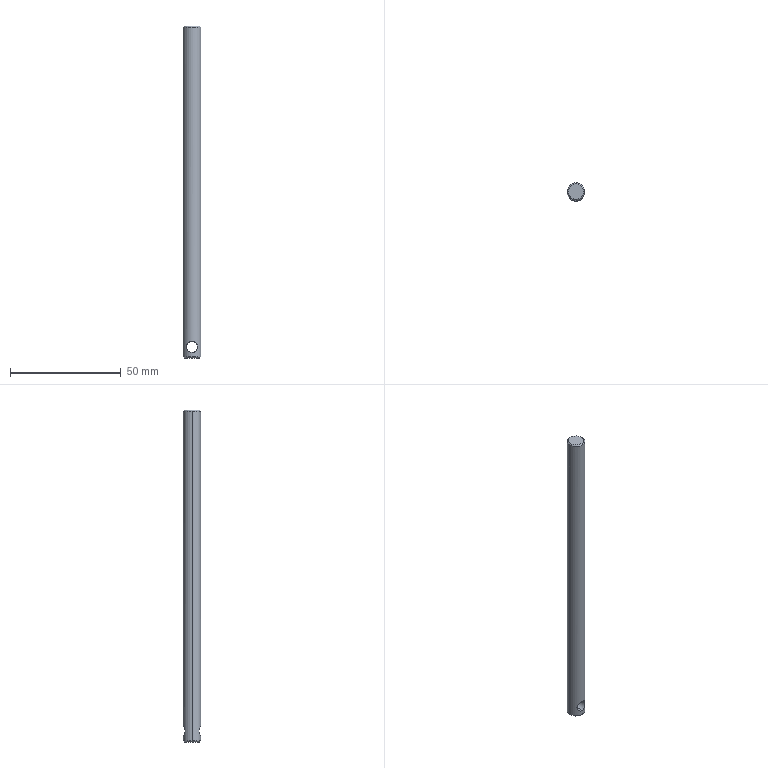Part | SolidWorks | features Chamfer 1, Extrusion 1, ICE 1 | 1 solid | 10 faces | box 8 x 8 x 150 mm | volume 7385 mm3 | cone 4 | cylinder 4 | plane 2 | commonest cylinder face diameters 5 x2 8 x2
STEP:
#1=CARTESIAN_POINT('',(-3.5,0.,-75.));
#2=VERTEX_POINT('',#1);
#3=CARTESIAN_POINT('',(3.5,0.,-75.));
#4=VERTEX_POINT('',#3);
#5=CARTESIAN_POINT('',(0.,0.,-75.));
#6=DIRECTION('',(0.,0.,-1.));
#7=DIRECTION('',(1.,0.,0.));
#8=AXIS2_PLACEMENT_3D('',#5,#6,#7);
#9=CIRCLE('',#8,3.5);
#10=EDGE_CURVE('',#2,#4,#9,.T.);
#11=ORIENTED_EDGE('',*,*,#10,.F.);
#12=CARTESIAN_POINT('',(-4.,0.,-74.5));
#13=VERTEX_POINT('',#12);
#14=CARTESIAN_POINT('',(-4.,0.,-74.5));
#15=DIRECTION('',(-0.7071,0.,0.7071));
#16=VECTOR('',#15,1000.);
#17=LINE('',#14,#16);
#18=EDGE_CURVE('',#2,#13,#17,.T.);
#19=ORIENTED_EDGE('',*,*,#18,.T.);
#20=CARTESIAN_POINT('',(4.,0.,-74.5));
#21=VERTEX_POINT('',#20);
#22=CARTESIAN_POINT('',(0.,0.,-74.5));
#23=DIRECTION('',(0.,0.,1.));
#24=DIRECTION('',(1.,0.,0.));
#25=AXIS2_PLACEMENT_3D('',#22,#23,#24);
#26=CIRCLE('',#25,4.);
#27=EDGE_CURVE('',#21,#13,#26,.T.);
#28=ORIENTED_EDGE('',*,*,#27,.F.);
#29=CARTESIAN_POINT('',(4.,0.,-74.5));
#30=DIRECTION('',(0.7071,0.,0.7071));
#31=VECTOR('',#30,1000.);
#32=LINE('',#29,#31);
#33=EDGE_CURVE('',#4,#21,#32,.T.);
#34=ORIENTED_EDGE('',*,*,#33,.F.);
#35=EDGE_LOOP('',(#11,#19,#28,#34));
#36=FACE_OUTER_BOUND('',#35,.T.);
#37=CARTESIAN_POINT('',(0.,0.,-74.5));
#38=DIRECTION('',(0.,0.,1.));
#39=DIRECTION('',(1.,0.,0.));
#40=AXIS2_PLACEMENT_3D('',#37,#38,#39);
#41=CONICAL_SURFACE('',#40,4.,0.7854);
#42=ADVANCED_FACE('',(#36),#41,.T.);
#43=CARTESIAN_POINT('',(3.5,0.,75.));
#44=VERTEX_POINT('',#43);
#45=CARTESIAN_POINT('',(-3.5,0.,75.));
#46=VERTEX_POINT('',#45);
#47=CARTESIAN_POINT('',(0.,0.,75.));
#48=DIRECTION('',(0.,0.,1.));
#49=DIRECTION('',(1.,0.,0.));
#50=AXIS2_PLACEMENT_3D('',#47,#48,#49);
#51=CIRCLE('',#50,3.5);
#52=EDGE_CURVE('',#44,#46,#51,.T.);
#53=ORIENTED_EDGE('',*,*,#52,.F.);
#54=CARTESIAN_POINT('',(4.,0.,74.5));
#55=VERTEX_POINT('',#54);
#56=CARTESIAN_POINT('',(3.5,0.,75.));
#57=DIRECTION('',(0.7071,0.,-0.7071));
#58=VECTOR('',#57,1000.);
#59=LINE('',#56,#58);
#60=EDGE_CURVE('',#44,#55,#59,.T.);
#61=ORIENTED_EDGE('',*,*,#60,.T.);
#62=CARTESIAN_POINT('',(-4.,0.,74.5));
#63=VERTEX_POINT('',#62);
#64=CARTESIAN_POINT('',(0.,0.,74.5));
#65=DIRECTION('',(0.,0.,-1.));
#66=DIRECTION('',(1.,0.,0.));
#67=AXIS2_PLACEMENT_3D('',#64,#65,#66);
#68=CIRCLE('',#67,4.);
#69=EDGE_CURVE('',#63,#55,#68,.T.);
#70=ORIENTED_EDGE('',*,*,#69,.F.);
#71=CARTESIAN_POINT('',(-3.5,0.,75.));
#72=DIRECTION('',(-0.7071,0.,-0.7071));
#73=VECTOR('',#72,1000.);
#74=LINE('',#71,#73);
#75=EDGE_CURVE('',#46,#63,#74,.T.);
#76=ORIENTED_EDGE('',*,*,#75,.F.);
#77=EDGE_LOOP('',(#53,#61,#70,#76));
#78=FACE_OUTER_BOUND('',#77,.T.);
#79=CARTESIAN_POINT('',(0.,0.,75.));
#80=DIRECTION('',(0.,0.,-1.));
#81=DIRECTION('',(-1.,0.,0.));
#82=AXIS2_PLACEMENT_3D('',#79,#80,#81);
#83=CONICAL_SURFACE('',#82,3.5,0.7854);
#84=ADVANCED_FACE('',(#78),#83,.T.);
#85=CARTESIAN_POINT('',(0.,-4.,-72.5));
#86=VERTEX_POINT('',#85);
#87=CARTESIAN_POINT('',(0.,-4.,-67.5));
#88=VERTEX_POINT('',#87);
#89=CARTESIAN_POINT('',(0.,-4.,-72.5));
#90=CARTESIAN_POINT('',(-0.1686,-4.,-72.5));
#91=CARTESIAN_POINT('',(-0.335,-3.989,-72.483));
#92=CARTESIAN_POINT('',(-0.6633,-3.948,-72.416));
#93=CARTESIAN_POINT('',(-0.8235,-3.917,-72.366));
#94=CARTESIAN_POINT('',(-1.125,-3.842,-72.239));
#95=CARTESIAN_POINT('',(-1.27,-3.796,-72.16));
#96=CARTESIAN_POINT('',(-1.536,-3.696,-71.979));
#97=CARTESIAN_POINT('',(-1.659,-3.642,-71.877));
#98=CARTESIAN_POINT('',(-1.884,-3.531,-71.651));
#99=CARTESIAN_POINT('',(-1.985,-3.474,-71.527));
#100=CARTESIAN_POINT('',(-2.163,-3.367,-71.264));
#101=CARTESIAN_POINT('',(-2.239,-3.315,-71.124));
#102=CARTESIAN_POINT('',(-2.367,-3.226,-70.822));
#103=CARTESIAN_POINT('',(-2.416,-3.189,-70.665));
#104=CARTESIAN_POINT('',(-2.482,-3.137,-70.34));
#105=CARTESIAN_POINT('',(-2.5,-3.123,-70.169));
#106=CARTESIAN_POINT('',(-2.5,-3.122,-69.834));
#107=CARTESIAN_POINT('',(-2.483,-3.136,-69.666));
#108=CARTESIAN_POINT('',(-2.416,-3.188,-69.337));
#109=CARTESIAN_POINT('',(-2.367,-3.225,-69.18));
#110=CARTESIAN_POINT('',(-2.177,-3.359,-68.729));
#111=CARTESIAN_POINT('',(-1.996,-3.476,-68.461));
#112=CARTESIAN_POINT('',(-1.659,-3.642,-68.123));
#113=CARTESIAN_POINT('',(-1.536,-3.696,-68.021));
#114=CARTESIAN_POINT('',(-1.271,-3.795,-67.841));
#115=CARTESIAN_POINT('',(-1.126,-3.841,-67.762));
#116=CARTESIAN_POINT('',(-0.8248,-3.917,-67.634));
#117=CARTESIAN_POINT('',(-0.6682,-3.947,-67.585));
#118=CARTESIAN_POINT('',(-0.3411,-3.989,-67.518));
#119=CARTESIAN_POINT('',(-0.1698,-4.,-67.5));
#120=CARTESIAN_POINT('',(0.,-4.,-67.5));
#121=B_SPLINE_CURVE_WITH_KNOTS('',3,(#89,#90,#91,#92,#93,#94,#95,#96,#97,#98,#99,#100,#101,#102,#103,#104,#105,#106,#107,#108,#109,#110,#111,#112,#113,#114,#115,#116,#117,#118,#119,#120),.UNSPECIFIED.,.F.,.F.,(4,2,2,2,2,2,2,2,2,2,2,2,2,2,2,4),(0.008042,0.008543,0.009045,0.009546,0.01005,0.01055,0.01105,0.01155,0.01205,0.01256,0.01306,0.01406,0.01456,0.01506,0.01556,0.01607),.UNSPECIFIED.);
#122=EDGE_CURVE('',#86,#88,#121,.T.);
#123=ORIENTED_EDGE('',*,*,#122,.F.);
#124=CARTESIAN_POINT('',(0.,4.,-72.5));
#125=VERTEX_POINT('',#124);
#126=CARTESIAN_POINT('',(0.,-75.,-72.5));
#127=DIRECTION('',(0.,1.,0.));
#128=VECTOR('',#127,1000.);
#129=LINE('',#126,#128);
#130=EDGE_CURVE('',#86,#125,#129,.T.);
#131=ORIENTED_EDGE('',*,*,#130,.T.);
#132=CARTESIAN_POINT('',(0.,4.,-67.5));
#133=VERTEX_POINT('',#132);
#134=CARTESIAN_POINT('',(0.,4.,-67.5));
#135=CARTESIAN_POINT('',(-0.1702,4.,-67.5));
#136=CARTESIAN_POINT('',(-0.3368,3.989,-67.517));
#137=CARTESIAN_POINT('',(-0.6632,3.948,-67.584));
#138=CARTESIAN_POINT('',(-0.8243,3.917,-67.634));
#139=CARTESIAN_POINT('',(-1.277,3.803,-67.826));
#140=CARTESIAN_POINT('',(-1.548,3.697,-68.011));
#141=CARTESIAN_POINT('',(-1.883,3.531,-68.348));
#142=CARTESIAN_POINT('',(-1.986,3.474,-68.473));
#143=CARTESIAN_POINT('',(-2.164,3.366,-68.737));
#144=CARTESIAN_POINT('',(-2.24,3.315,-68.877));
#145=CARTESIAN_POINT('',(-2.366,3.226,-69.175));
#146=CARTESIAN_POINT('',(-2.416,3.188,-69.335));
#147=CARTESIAN_POINT('',(-2.482,3.137,-69.661));
#148=CARTESIAN_POINT('',(-2.5,3.123,-69.83));
#149=CARTESIAN_POINT('',(-2.5,3.122,-70.169));
#150=CARTESIAN_POINT('',(-2.483,3.136,-70.335));
#151=CARTESIAN_POINT('',(-2.416,3.188,-70.662));
#152=CARTESIAN_POINT('',(-2.367,3.226,-70.821));
#153=CARTESIAN_POINT('',(-2.24,3.315,-71.121));
#154=CARTESIAN_POINT('',(-2.163,3.367,-71.264));
#155=CARTESIAN_POINT('',(-1.984,3.475,-71.529));
#156=CARTESIAN_POINT('',(-1.883,3.531,-71.652));
#157=CARTESIAN_POINT('',(-1.545,3.698,-71.992));
#158=CARTESIAN_POINT('',(-1.28,3.803,-72.173));
#159=CARTESIAN_POINT('',(-0.8216,3.918,-72.367));
#160=CARTESIAN_POINT('',(-0.664,3.948,-72.416));
#161=CARTESIAN_POINT('',(-0.339,3.989,-72.482));
#162=CARTESIAN_POINT('',(-0.169,4.,-72.5));
#163=CARTESIAN_POINT('',(0.,4.,-72.5));
#164=B_SPLINE_CURVE_WITH_KNOTS('',3,(#134,#135,#136,#137,#138,#139,#140,#141,#142,#143,#144,#145,#146,#147,#148,#149,#150,#151,#152,#153,#154,#155,#156,#157,#158,#159,#160,#161,#162,#163),.UNSPECIFIED.,.F.,.F.,(4,2,2,2,2,2,2,2,2,2,2,2,2,2,4),(0.,0.0005026,0.001005,0.002011,0.002513,0.003016,0.003518,0.004021,0.004524,0.005026,0.005529,0.006032,0.007037,0.007539,0.008042),.UNSPECIFIED.);
#165=EDGE_CURVE('',#133,#125,#164,.T.);
#166=ORIENTED_EDGE('',*,*,#165,.F.);
#167=CARTESIAN_POINT('',(0.,-75.,-67.5));
#168=DIRECTION('',(0.,1.,0.));
#169=VECTOR('',#168,1000.);
#170=LINE('',#167,#169);
#171=EDGE_CURVE('',#88,#133,#170,.T.);
#172=ORIENTED_EDGE('',*,*,#171,.F.);
#173=EDGE_LOOP('',(#123,#131,#166,#172));
#174=FACE_OUTER_BOUND('',#173,.T.);
#175=CARTESIAN_POINT('',(0.,-75.,-70.));
#176=DIRECTION('',(0.,1.,0.));
#177=DIRECTION('',(0.,0.,1.));
#178=AXIS2_PLACEMENT_3D('',#175,#176,#177);
#179=CYLINDRICAL_SURFACE('',#178,2.5);
#180=ADVANCED_FACE('',(#174),#179,.F.);
#181=ORIENTED_EDGE('',*,*,#165,.T.);
#182=CARTESIAN_POINT('',(0.,4.,-72.5));
#183=CARTESIAN_POINT('',(0.1686,4.,-72.5));
#184=CARTESIAN_POINT('',(0.335,3.989,-72.483));
#185=CARTESIAN_POINT('',(0.6633,3.948,-72.416));
#186=CARTESIAN_POINT('',(0.8235,3.917,-72.366));
#187=CARTESIAN_POINT('',(1.125,3.842,-72.239));
#188=CARTESIAN_POINT('',(1.27,3.796,-72.16));
#189=CARTESIAN_POINT('',(1.536,3.696,-71.979));
#190=CARTESIAN_POINT('',(1.659,3.642,-71.877));
#191=CARTESIAN_POINT('',(1.884,3.531,-71.651));
#192=CARTESIAN_POINT('',(1.985,3.474,-71.527));
#193=CARTESIAN_POINT('',(2.163,3.367,-71.264));
#194=CARTESIAN_POINT('',(2.239,3.315,-71.124));
#195=CARTESIAN_POINT('',(2.367,3.226,-70.822));
#196=CARTESIAN_POINT('',(2.416,3.189,-70.665));
#197=CARTESIAN_POINT('',(2.482,3.137,-70.34));
#198=CARTESIAN_POINT('',(2.5,3.123,-70.169));
#199=CARTESIAN_POINT('',(2.5,3.122,-69.834));
#200=CARTESIAN_POINT('',(2.483,3.136,-69.666));
#201=CARTESIAN_POINT('',(2.416,3.188,-69.337));
#202=CARTESIAN_POINT('',(2.367,3.225,-69.18));
#203=CARTESIAN_POINT('',(2.177,3.359,-68.729));
#204=CARTESIAN_POINT('',(1.996,3.476,-68.461));
#205=CARTESIAN_POINT('',(1.659,3.642,-68.123));
#206=CARTESIAN_POINT('',(1.536,3.696,-68.021));
#207=CARTESIAN_POINT('',(1.271,3.795,-67.841));
#208=CARTESIAN_POINT('',(1.126,3.841,-67.762));
#209=CARTESIAN_POINT('',(0.8248,3.917,-67.634));
#210=CARTESIAN_POINT('',(0.6682,3.947,-67.585));
#211=CARTESIAN_POINT('',(0.3411,3.989,-67.518));
#212=CARTESIAN_POINT('',(0.1698,4.,-67.5));
#213=CARTESIAN_POINT('',(0.,4.,-67.5));
#214=B_SPLINE_CURVE_WITH_KNOTS('',3,(#182,#183,#184,#185,#186,#187,#188,#189,#190,#191,#192,#193,#194,#195,#196,#197,#198,#199,#200,#201,#202,#203,#204,#205,#206,#207,#208,#209,#210,#211,#212,#213),.UNSPECIFIED.,.F.,.F.,(4,2,2,2,2,2,2,2,2,2,2,2,2,2,2,4),(0.008042,0.008543,0.009045,0.009546,0.01005,0.01055,0.01105,0.01155,0.01205,0.01256,0.01306,0.01406,0.01456,0.01506,0.01556,0.01607),.UNSPECIFIED.);
#215=EDGE_CURVE('',#125,#133,#214,.T.);
#216=ORIENTED_EDGE('',*,*,#215,.T.);
#217=EDGE_LOOP('',(#181,#216));
#218=FACE_BOUND('',#217,.T.);
#219=ORIENTED_EDGE('',*,*,#69,.T.);
#220=CARTESIAN_POINT('',(4.,0.,75.));
#221=DIRECTION('',(0.,0.,-1.));
#222=VECTOR('',#221,1000.);
#223=LINE('',#220,#222);
#224=EDGE_CURVE('',#55,#21,#223,.T.);
#225=ORIENTED_EDGE('',*,*,#224,.T.);
#226=ORIENTED_EDGE('',*,*,#27,.T.);
#227=CARTESIAN_POINT('',(-4.,0.,75.));
#228=DIRECTION('',(0.,0.,-1.));
#229=VECTOR('',#228,1000.);
#230=LINE('',#227,#229);
#231=EDGE_CURVE('',#63,#13,#230,.T.);
#232=ORIENTED_EDGE('',*,*,#231,.F.);
#233=EDGE_LOOP('',(#219,#225,#226,#232));
#234=FACE_OUTER_BOUND('',#233,.T.);
#235=CARTESIAN_POINT('',(0.,0.,75.));
#236=DIRECTION('',(0.,0.,-1.));
#237=DIRECTION('',(-1.,0.,0.));
#238=AXIS2_PLACEMENT_3D('',#235,#236,#237);
#239=CYLINDRICAL_SURFACE('',#238,4.);
#240=ADVANCED_FACE('',(#218,#234),#239,.T.);
#241=ORIENTED_EDGE('',*,*,#224,.F.);
#242=CARTESIAN_POINT('',(0.,0.,74.5));
#243=DIRECTION('',(0.,0.,-1.));
#244=DIRECTION('',(1.,0.,0.));
#245=AXIS2_PLACEMENT_3D('',#242,#243,#244);
#246=CIRCLE('',#245,4.);
#247=EDGE_CURVE('',#55,#63,#246,.T.);
#248=ORIENTED_EDGE('',*,*,#247,.T.);
#249=ORIENTED_EDGE('',*,*,#231,.T.);
#250=CARTESIAN_POINT('',(0.,0.,-74.5));
#251=DIRECTION('',(0.,0.,1.));
#252=DIRECTION('',(1.,0.,0.));
#253=AXIS2_PLACEMENT_3D('',#250,#251,#252);
#254=CIRCLE('',#253,4.);
#255=EDGE_CURVE('',#13,#21,#254,.T.);
#256=ORIENTED_EDGE('',*,*,#255,.T.);
#257=EDGE_LOOP('',(#241,#248,#249,#256));
#258=FACE_OUTER_BOUND('',#257,.T.);
#259=CARTESIAN_POINT('',(0.,-4.,-67.5));
#260=CARTESIAN_POINT('',(0.1702,-4.,-67.5));
#261=CARTESIAN_POINT('',(0.3368,-3.989,-67.517));
#262=CARTESIAN_POINT('',(0.6632,-3.948,-67.584));
#263=CARTESIAN_POINT('',(0.8243,-3.917,-67.634));
#264=CARTESIAN_POINT('',(1.277,-3.803,-67.826));
#265=CARTESIAN_POINT('',(1.548,-3.697,-68.011));
#266=CARTESIAN_POINT('',(1.883,-3.531,-68.348));
#267=CARTESIAN_POINT('',(1.986,-3.474,-68.473));
#268=CARTESIAN_POINT('',(2.164,-3.366,-68.737));
#269=CARTESIAN_POINT('',(2.24,-3.315,-68.877));
#270=CARTESIAN_POINT('',(2.366,-3.226,-69.175));
#271=CARTESIAN_POINT('',(2.416,-3.188,-69.335));
#272=CARTESIAN_POINT('',(2.482,-3.137,-69.661));
#273=CARTESIAN_POINT('',(2.5,-3.123,-69.83));
#274=CARTESIAN_POINT('',(2.5,-3.122,-70.169));
#275=CARTESIAN_POINT('',(2.483,-3.136,-70.335));
#276=CARTESIAN_POINT('',(2.416,-3.188,-70.662));
#277=CARTESIAN_POINT('',(2.367,-3.226,-70.821));
#278=CARTESIAN_POINT('',(2.24,-3.315,-71.121));
#279=CARTESIAN_POINT('',(2.163,-3.367,-71.264));
#280=CARTESIAN_POINT('',(1.984,-3.475,-71.529));
#281=CARTESIAN_POINT('',(1.883,-3.531,-71.652));
#282=CARTESIAN_POINT('',(1.545,-3.698,-71.992));
#283=CARTESIAN_POINT('',(1.28,-3.803,-72.173));
#284=CARTESIAN_POINT('',(0.8216,-3.918,-72.367));
#285=CARTESIAN_POINT('',(0.664,-3.948,-72.416));
#286=CARTESIAN_POINT('',(0.339,-3.989,-72.482));
#287=CARTESIAN_POINT('',(0.169,-4.,-72.5));
#288=CARTESIAN_POINT('',(0.,-4.,-72.5));
#289=B_SPLINE_CURVE_WITH_KNOTS('',3,(#259,#260,#261,#262,#263,#264,#265,#266,#267,#268,#269,#270,#271,#272,#273,#274,#275,#276,#277,#278,#279,#280,#281,#282,#283,#284,#285,#286,#287,#288),.UNSPECIFIED.,.F.,.F.,(4,2,2,2,2,2,2,2,2,2,2,2,2,2,4),(0.,0.0005026,0.001005,0.002011,0.002513,0.003016,0.003518,0.004021,0.004524,0.005026,0.005529,0.006032,0.007037,0.007539,0.008042),.UNSPECIFIED.);
#290=EDGE_CURVE('',#88,#86,#289,.T.);
#291=ORIENTED_EDGE('',*,*,#290,.T.);
#292=ORIENTED_EDGE('',*,*,#122,.T.);
#293=EDGE_LOOP('',(#291,#292));
#294=FACE_BOUND('',#293,.T.);
#295=CARTESIAN_POINT('',(0.,0.,75.));
#296=DIRECTION('',(0.,0.,-1.));
#297=DIRECTION('',(-1.,0.,0.));
#298=AXIS2_PLACEMENT_3D('',#295,#296,#297);
#299=CYLINDRICAL_SURFACE('',#298,4.);
#300=ADVANCED_FACE('',(#258,#294),#299,.T.);
#301=CARTESIAN_POINT('',(0.,0.,75.));
#302=DIRECTION('',(0.,0.,1.));
#303=DIRECTION('',(1.,0.,0.));
#304=AXIS2_PLACEMENT_3D('',#301,#302,#303);
#305=CIRCLE('',#304,3.5);
#306=EDGE_CURVE('',#46,#44,#305,.T.);
#307=ORIENTED_EDGE('',*,*,#306,.T.);
#308=ORIENTED_EDGE('',*,*,#52,.T.);
#309=EDGE_LOOP('',(#307,#308));
#310=FACE_OUTER_BOUND('',#309,.T.);
#311=CARTESIAN_POINT('',(0.,0.,75.));
#312=DIRECTION('',(0.,0.,1.));
#313=DIRECTION('',(1.,0.,0.));
#314=AXIS2_PLACEMENT_3D('',#311,#312,#313);
#315=PLANE('',#314);
#316=ADVANCED_FACE('',(#310),#315,.T.);
#317=CARTESIAN_POINT('',(0.,0.,-75.));
#318=DIRECTION('',(0.,0.,-1.));
#319=DIRECTION('',(1.,0.,0.));
#320=AXIS2_PLACEMENT_3D('',#317,#318,#319);
#321=CIRCLE('',#320,3.5);
#322=EDGE_CURVE('',#4,#2,#321,.T.);
#323=ORIENTED_EDGE('',*,*,#322,.T.);
#324=ORIENTED_EDGE('',*,*,#10,.T.);
#325=EDGE_LOOP('',(#323,#324));
#326=FACE_OUTER_BOUND('',#325,.T.);
#327=CARTESIAN_POINT('',(0.,0.,-75.));
#328=DIRECTION('',(0.,0.,1.));
#329=DIRECTION('',(1.,0.,0.));
#330=AXIS2_PLACEMENT_3D('',#327,#328,#329);
#331=PLANE('',#330);
#332=ADVANCED_FACE('',(#326),#331,.F.);
#333=ORIENTED_EDGE('',*,*,#130,.F.);
#334=ORIENTED_EDGE('',*,*,#290,.F.);
#335=ORIENTED_EDGE('',*,*,#171,.T.);
#336=ORIENTED_EDGE('',*,*,#215,.F.);
#337=EDGE_LOOP('',(#333,#334,#335,#336));
#338=FACE_OUTER_BOUND('',#337,.T.);
#339=CARTESIAN_POINT('',(0.,-75.,-70.));
#340=DIRECTION('',(0.,1.,0.));
#341=DIRECTION('',(0.,0.,1.));
#342=AXIS2_PLACEMENT_3D('',#339,#340,#341);
#343=CYLINDRICAL_SURFACE('',#342,2.5);
#344=ADVANCED_FACE('',(#338),#343,.F.);
#345=ORIENTED_EDGE('',*,*,#60,.F.);
#346=ORIENTED_EDGE('',*,*,#306,.F.);
#347=ORIENTED_EDGE('',*,*,#75,.T.);
#348=ORIENTED_EDGE('',*,*,#247,.F.);
#349=EDGE_LOOP('',(#345,#346,#347,#348));
#350=FACE_OUTER_BOUND('',#349,.T.);
#351=CARTESIAN_POINT('',(0.,0.,75.));
#352=DIRECTION('',(0.,0.,-1.));
#353=DIRECTION('',(-1.,0.,0.));
#354=AXIS2_PLACEMENT_3D('',#351,#352,#353);
#355=CONICAL_SURFACE('',#354,3.5,0.7854);
#356=ADVANCED_FACE('',(#350),#355,.T.);
#357=ORIENTED_EDGE('',*,*,#18,.F.);
#358=ORIENTED_EDGE('',*,*,#322,.F.);
#359=ORIENTED_EDGE('',*,*,#33,.T.);
#360=ORIENTED_EDGE('',*,*,#255,.F.);
#361=EDGE_LOOP('',(#357,#358,#359,#360));
#362=FACE_OUTER_BOUND('',#361,.T.);
#363=CARTESIAN_POINT('',(0.,0.,-74.5));
#364=DIRECTION('',(0.,0.,1.));
#365=DIRECTION('',(1.,0.,0.));
#366=AXIS2_PLACEMENT_3D('',#363,#364,#365);
#367=CONICAL_SURFACE('',#366,4.,0.7854);
#368=ADVANCED_FACE('',(#362),#367,.T.);
#369=CLOSED_SHELL('',(#42,#84,#180,#240,#300,#316,#332,#344,#356,#368));
#370=MANIFOLD_SOLID_BREP('',#369);
#371=CARTESIAN_POINT('',(0.,0.,0.));
#372=DIRECTION('',(0.,0.,1.));
#373=DIRECTION('',(1.,0.,0.));
#374=AXIS2_PLACEMENT_3D('',#371,#372,#373);
#375=(LENGTH_UNIT()NAMED_UNIT(*)SI_UNIT(.MILLI.,.METRE.));
#376=UNCERTAINTY_MEASURE_WITH_UNIT(LENGTH_MEASURE(0.00001),#375,'','');
#377=(NAMED_UNIT(*)PLANE_ANGLE_UNIT()SI_UNIT($,.RADIAN.));
#378=(NAMED_UNIT(*)SI_UNIT($,.STERADIAN.)SOLID_ANGLE_UNIT());
#379=(GEOMETRIC_REPRESENTATION_CONTEXT(3)GLOBAL_UNCERTAINTY_ASSIGNED_CONTEXT((#376))GLOBAL_UNIT_ASSIGNED_CONTEXT((#375,#377,#378))REPRESENTATION_CONTEXT('',''));
#380=ADVANCED_BREP_SHAPE_REPRESENTATION('',(#370,#374),#379);